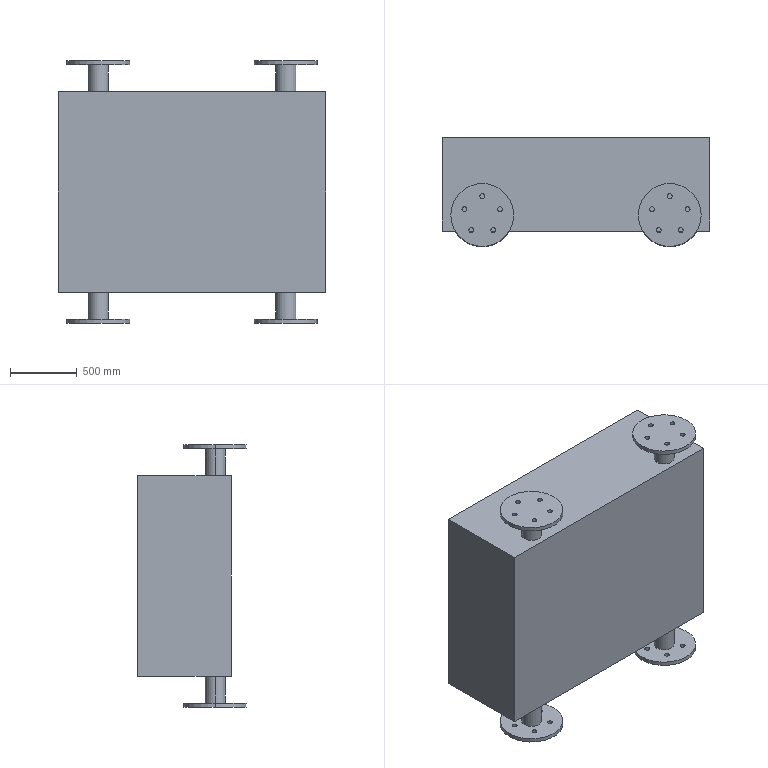Part | SolidWorks | features BaseBody 4 | 4 solids | 76 faces | box 2000 x 815 x 1960 mm | volume 2130497325 mm3 | cylinder 58 | plane 18 | commonest cylinder face diameters 36 x40 150 x8 470 x8 700 x2